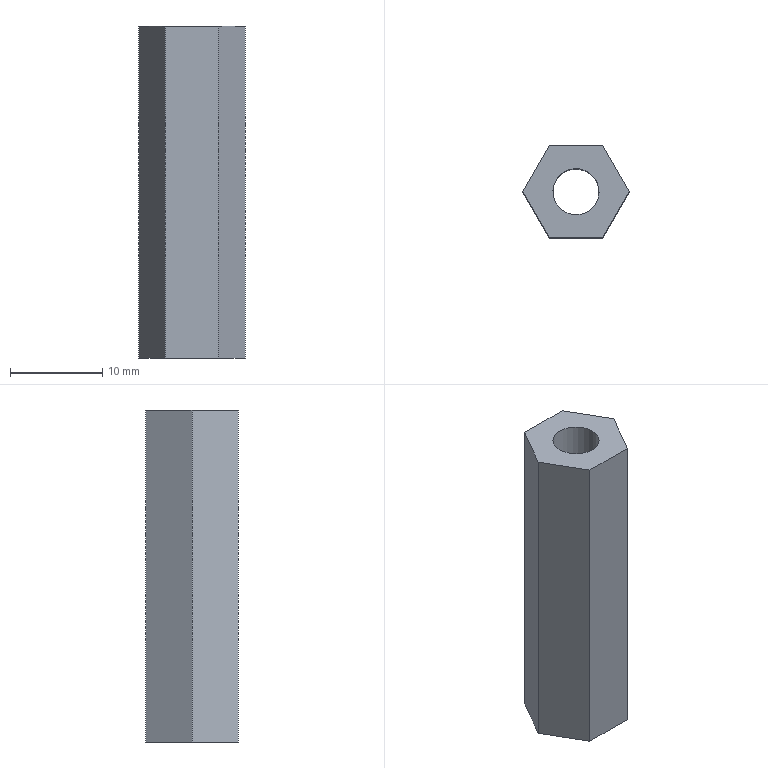Part | NX | features BREP 1 | 1 solid | 10 faces | box 11.547 x 10 x 36 mm | volume 2411 mm3 | plane 8 | cylinder 2 | commonest cylinder face diameters 5 x2
STEP:
#1=CARTESIAN_POINT('',(-121.835,201.259,18.));
#2=VERTEX_POINT('',#1);
#3=CARTESIAN_POINT('',(-126.165,203.759,18.));
#4=VERTEX_POINT('',#3);
#5=CARTESIAN_POINT('',(-124.,202.509,18.));
#6=DIRECTION('',(0.,0.,1.));
#7=DIRECTION('',(-0.866,0.5,0.));
#8=AXIS2_PLACEMENT_3D('',#5,#6,#7);
#9=CIRCLE('',#8,2.5);
#10=EDGE_CURVE('',#2,#4,#9,.T.);
#11=ORIENTED_EDGE('',*,*,#10,.T.);
#12=CARTESIAN_POINT('',(-126.165,203.759,-18.));
#13=VERTEX_POINT('',#12);
#14=CARTESIAN_POINT('',(-126.165,203.759,18.));
#15=DIRECTION('',(0.,0.,1.));
#16=VECTOR('',#15,1000.);
#17=LINE('',#14,#16);
#18=EDGE_CURVE('',#13,#4,#17,.T.);
#19=ORIENTED_EDGE('',*,*,#18,.F.);
#20=CARTESIAN_POINT('',(-121.835,201.259,-18.));
#21=VERTEX_POINT('',#20);
#22=CARTESIAN_POINT('',(-124.,202.509,-18.));
#23=DIRECTION('',(0.,0.,1.));
#24=DIRECTION('',(-0.866,0.5,0.));
#25=AXIS2_PLACEMENT_3D('',#22,#23,#24);
#26=CIRCLE('',#25,2.5);
#27=EDGE_CURVE('',#21,#13,#26,.T.);
#28=ORIENTED_EDGE('',*,*,#27,.F.);
#29=CARTESIAN_POINT('',(-121.835,201.259,18.));
#30=DIRECTION('',(0.,0.,-1.));
#31=VECTOR('',#30,1000.);
#32=LINE('',#29,#31);
#33=EDGE_CURVE('',#2,#21,#32,.T.);
#34=ORIENTED_EDGE('',*,*,#33,.F.);
#35=EDGE_LOOP('',(#11,#19,#28,#34));
#36=FACE_BOUND('',#35,.T.);
#37=CARTESIAN_POINT('',(-124.,202.509,18.));
#38=DIRECTION('',(0.,0.,-1.));
#39=DIRECTION('',(-0.866,0.5,0.));
#40=AXIS2_PLACEMENT_3D('',#37,#38,#39);
#41=CYLINDRICAL_SURFACE('',#40,2.5);
#42=ADVANCED_FACE('',(#36),#41,.F.);
#43=CARTESIAN_POINT('',(-126.887,207.509,18.));
#44=VERTEX_POINT('',#43);
#45=CARTESIAN_POINT('',(-129.774,202.509,18.));
#46=VERTEX_POINT('',#45);
#47=CARTESIAN_POINT('',(-126.887,207.509,18.));
#48=DIRECTION('',(-0.5,-0.866,0.));
#49=VECTOR('',#48,1000.);
#50=LINE('',#47,#49);
#51=EDGE_CURVE('',#44,#46,#50,.T.);
#52=ORIENTED_EDGE('',*,*,#51,.T.);
#53=CARTESIAN_POINT('',(-126.887,197.509,18.));
#54=VERTEX_POINT('',#53);
#55=CARTESIAN_POINT('',(-129.774,202.509,18.));
#56=DIRECTION('',(0.5,-0.866,0.));
#57=VECTOR('',#56,1000.);
#58=LINE('',#55,#57);
#59=EDGE_CURVE('',#46,#54,#58,.T.);
#60=ORIENTED_EDGE('',*,*,#59,.T.);
#61=CARTESIAN_POINT('',(-121.113,197.509,18.));
#62=VERTEX_POINT('',#61);
#63=CARTESIAN_POINT('',(-126.887,197.509,18.));
#64=DIRECTION('',(1.,0.,0.));
#65=VECTOR('',#64,1000.);
#66=LINE('',#63,#65);
#67=EDGE_CURVE('',#54,#62,#66,.T.);
#68=ORIENTED_EDGE('',*,*,#67,.T.);
#69=CARTESIAN_POINT('',(-118.226,202.509,18.));
#70=VERTEX_POINT('',#69);
#71=CARTESIAN_POINT('',(-121.113,197.509,18.));
#72=DIRECTION('',(0.5,0.866,0.));
#73=VECTOR('',#72,1000.);
#74=LINE('',#71,#73);
#75=EDGE_CURVE('',#62,#70,#74,.T.);
#76=ORIENTED_EDGE('',*,*,#75,.T.);
#77=CARTESIAN_POINT('',(-121.113,207.509,18.));
#78=VERTEX_POINT('',#77);
#79=CARTESIAN_POINT('',(-118.226,202.509,18.));
#80=DIRECTION('',(-0.5,0.866,0.));
#81=VECTOR('',#80,1000.);
#82=LINE('',#79,#81);
#83=EDGE_CURVE('',#70,#78,#82,.T.);
#84=ORIENTED_EDGE('',*,*,#83,.T.);
#85=CARTESIAN_POINT('',(-121.113,207.509,18.));
#86=DIRECTION('',(-1.,0.,0.));
#87=VECTOR('',#86,1000.);
#88=LINE('',#85,#87);
#89=EDGE_CURVE('',#78,#44,#88,.T.);
#90=ORIENTED_EDGE('',*,*,#89,.T.);
#91=EDGE_LOOP('',(#52,#60,#68,#76,#84,#90));
#92=FACE_BOUND('',#91,.T.);
#93=ORIENTED_EDGE('',*,*,#10,.F.);
#94=CARTESIAN_POINT('',(-124.,202.509,18.));
#95=DIRECTION('',(0.,0.,1.));
#96=DIRECTION('',(-0.866,0.5,0.));
#97=AXIS2_PLACEMENT_3D('',#94,#95,#96);
#98=CIRCLE('',#97,2.5);
#99=EDGE_CURVE('',#4,#2,#98,.T.);
#100=ORIENTED_EDGE('',*,*,#99,.F.);
#101=EDGE_LOOP('',(#93,#100));
#102=FACE_BOUND('',#101,.T.);
#103=CARTESIAN_POINT('',(-124.,202.509,18.));
#104=DIRECTION('',(0.,0.,1.));
#105=DIRECTION('',(0.866,-0.5,0.));
#106=AXIS2_PLACEMENT_3D('',#103,#104,#105);
#107=PLANE('',#106);
#108=ADVANCED_FACE('',(#92,#102),#107,.T.);
#109=CARTESIAN_POINT('',(-126.887,207.509,-18.));
#110=VERTEX_POINT('',#109);
#111=CARTESIAN_POINT('',(-129.774,202.509,-18.));
#112=VERTEX_POINT('',#111);
#113=CARTESIAN_POINT('',(-126.887,207.509,-18.));
#114=DIRECTION('',(-0.5,-0.866,0.));
#115=VECTOR('',#114,1000.);
#116=LINE('',#113,#115);
#117=EDGE_CURVE('',#110,#112,#116,.T.);
#118=ORIENTED_EDGE('',*,*,#117,.F.);
#119=CARTESIAN_POINT('',(-121.113,207.509,-18.));
#120=VERTEX_POINT('',#119);
#121=CARTESIAN_POINT('',(-121.113,207.509,-18.));
#122=DIRECTION('',(-1.,0.,0.));
#123=VECTOR('',#122,1000.);
#124=LINE('',#121,#123);
#125=EDGE_CURVE('',#120,#110,#124,.T.);
#126=ORIENTED_EDGE('',*,*,#125,.F.);
#127=CARTESIAN_POINT('',(-118.226,202.509,-18.));
#128=VERTEX_POINT('',#127);
#129=CARTESIAN_POINT('',(-118.226,202.509,-18.));
#130=DIRECTION('',(-0.5,0.866,0.));
#131=VECTOR('',#130,1000.);
#132=LINE('',#129,#131);
#133=EDGE_CURVE('',#128,#120,#132,.T.);
#134=ORIENTED_EDGE('',*,*,#133,.F.);
#135=CARTESIAN_POINT('',(-121.113,197.509,-18.));
#136=VERTEX_POINT('',#135);
#137=CARTESIAN_POINT('',(-121.113,197.509,-18.));
#138=DIRECTION('',(0.5,0.866,0.));
#139=VECTOR('',#138,1000.);
#140=LINE('',#137,#139);
#141=EDGE_CURVE('',#136,#128,#140,.T.);
#142=ORIENTED_EDGE('',*,*,#141,.F.);
#143=CARTESIAN_POINT('',(-126.887,197.509,-18.));
#144=VERTEX_POINT('',#143);
#145=CARTESIAN_POINT('',(-126.887,197.509,-18.));
#146=DIRECTION('',(1.,0.,0.));
#147=VECTOR('',#146,1000.);
#148=LINE('',#145,#147);
#149=EDGE_CURVE('',#144,#136,#148,.T.);
#150=ORIENTED_EDGE('',*,*,#149,.F.);
#151=CARTESIAN_POINT('',(-129.774,202.509,-18.));
#152=DIRECTION('',(0.5,-0.866,0.));
#153=VECTOR('',#152,1000.);
#154=LINE('',#151,#153);
#155=EDGE_CURVE('',#112,#144,#154,.T.);
#156=ORIENTED_EDGE('',*,*,#155,.F.);
#157=EDGE_LOOP('',(#118,#126,#134,#142,#150,#156));
#158=FACE_BOUND('',#157,.T.);
#159=ORIENTED_EDGE('',*,*,#27,.T.);
#160=CARTESIAN_POINT('',(-124.,202.509,-18.));
#161=DIRECTION('',(0.,0.,1.));
#162=DIRECTION('',(-0.866,0.5,0.));
#163=AXIS2_PLACEMENT_3D('',#160,#161,#162);
#164=CIRCLE('',#163,2.5);
#165=EDGE_CURVE('',#13,#21,#164,.T.);
#166=ORIENTED_EDGE('',*,*,#165,.T.);
#167=EDGE_LOOP('',(#159,#166));
#168=FACE_BOUND('',#167,.T.);
#169=CARTESIAN_POINT('',(-124.,202.509,-18.));
#170=DIRECTION('',(0.,0.,1.));
#171=DIRECTION('',(0.866,-0.5,0.));
#172=AXIS2_PLACEMENT_3D('',#169,#170,#171);
#173=PLANE('',#172);
#174=ADVANCED_FACE('',(#158,#168),#173,.F.);
#175=ORIENTED_EDGE('',*,*,#117,.T.);
#176=CARTESIAN_POINT('',(-129.774,202.509,18.));
#177=DIRECTION('',(0.,0.,-1.));
#178=VECTOR('',#177,1000.);
#179=LINE('',#176,#178);
#180=EDGE_CURVE('',#46,#112,#179,.T.);
#181=ORIENTED_EDGE('',*,*,#180,.F.);
#182=ORIENTED_EDGE('',*,*,#51,.F.);
#183=CARTESIAN_POINT('',(-126.887,207.509,18.));
#184=DIRECTION('',(0.,0.,-1.));
#185=VECTOR('',#184,1000.);
#186=LINE('',#183,#185);
#187=EDGE_CURVE('',#44,#110,#186,.T.);
#188=ORIENTED_EDGE('',*,*,#187,.T.);
#189=EDGE_LOOP('',(#175,#181,#182,#188));
#190=FACE_BOUND('',#189,.T.);
#191=CARTESIAN_POINT('',(-126.887,207.509,18.));
#192=DIRECTION('',(0.866,-0.5,0.));
#193=DIRECTION('',(-0.5,-0.866,0.));
#194=AXIS2_PLACEMENT_3D('',#191,#192,#193);
#195=PLANE('',#194);
#196=ADVANCED_FACE('',(#190),#195,.F.);
#197=ORIENTED_EDGE('',*,*,#155,.T.);
#198=CARTESIAN_POINT('',(-126.887,197.509,18.));
#199=DIRECTION('',(0.,0.,-1.));
#200=VECTOR('',#199,1000.);
#201=LINE('',#198,#200);
#202=EDGE_CURVE('',#54,#144,#201,.T.);
#203=ORIENTED_EDGE('',*,*,#202,.F.);
#204=ORIENTED_EDGE('',*,*,#59,.F.);
#205=ORIENTED_EDGE('',*,*,#180,.T.);
#206=EDGE_LOOP('',(#197,#203,#204,#205));
#207=FACE_BOUND('',#206,.T.);
#208=CARTESIAN_POINT('',(-129.774,202.509,18.));
#209=DIRECTION('',(0.866,0.5,0.));
#210=DIRECTION('',(0.5,-0.866,0.));
#211=AXIS2_PLACEMENT_3D('',#208,#209,#210);
#212=PLANE('',#211);
#213=ADVANCED_FACE('',(#207),#212,.F.);
#214=ORIENTED_EDGE('',*,*,#149,.T.);
#215=CARTESIAN_POINT('',(-121.113,197.509,18.));
#216=DIRECTION('',(0.,0.,-1.));
#217=VECTOR('',#216,1000.);
#218=LINE('',#215,#217);
#219=EDGE_CURVE('',#62,#136,#218,.T.);
#220=ORIENTED_EDGE('',*,*,#219,.F.);
#221=ORIENTED_EDGE('',*,*,#67,.F.);
#222=ORIENTED_EDGE('',*,*,#202,.T.);
#223=EDGE_LOOP('',(#214,#220,#221,#222));
#224=FACE_BOUND('',#223,.T.);
#225=CARTESIAN_POINT('',(-126.887,197.509,18.));
#226=DIRECTION('',(0.,1.,0.));
#227=DIRECTION('',(1.,0.,0.));
#228=AXIS2_PLACEMENT_3D('',#225,#226,#227);
#229=PLANE('',#228);
#230=ADVANCED_FACE('',(#224),#229,.F.);
#231=ORIENTED_EDGE('',*,*,#141,.T.);
#232=CARTESIAN_POINT('',(-118.226,202.509,18.));
#233=DIRECTION('',(0.,0.,-1.));
#234=VECTOR('',#233,1000.);
#235=LINE('',#232,#234);
#236=EDGE_CURVE('',#70,#128,#235,.T.);
#237=ORIENTED_EDGE('',*,*,#236,.F.);
#238=ORIENTED_EDGE('',*,*,#75,.F.);
#239=ORIENTED_EDGE('',*,*,#219,.T.);
#240=EDGE_LOOP('',(#231,#237,#238,#239));
#241=FACE_BOUND('',#240,.T.);
#242=CARTESIAN_POINT('',(-121.113,197.509,18.));
#243=DIRECTION('',(-0.866,0.5,0.));
#244=DIRECTION('',(0.5,0.866,0.));
#245=AXIS2_PLACEMENT_3D('',#242,#243,#244);
#246=PLANE('',#245);
#247=ADVANCED_FACE('',(#241),#246,.F.);
#248=ORIENTED_EDGE('',*,*,#133,.T.);
#249=CARTESIAN_POINT('',(-121.113,207.509,18.));
#250=DIRECTION('',(0.,0.,-1.));
#251=VECTOR('',#250,1000.);
#252=LINE('',#249,#251);
#253=EDGE_CURVE('',#78,#120,#252,.T.);
#254=ORIENTED_EDGE('',*,*,#253,.F.);
#255=ORIENTED_EDGE('',*,*,#83,.F.);
#256=ORIENTED_EDGE('',*,*,#236,.T.);
#257=EDGE_LOOP('',(#248,#254,#255,#256));
#258=FACE_BOUND('',#257,.T.);
#259=CARTESIAN_POINT('',(-118.226,202.509,18.));
#260=DIRECTION('',(-0.866,-0.5,0.));
#261=DIRECTION('',(-0.5,0.866,0.));
#262=AXIS2_PLACEMENT_3D('',#259,#260,#261);
#263=PLANE('',#262);
#264=ADVANCED_FACE('',(#258),#263,.F.);
#265=ORIENTED_EDGE('',*,*,#125,.T.);
#266=ORIENTED_EDGE('',*,*,#187,.F.);
#267=ORIENTED_EDGE('',*,*,#89,.F.);
#268=ORIENTED_EDGE('',*,*,#253,.T.);
#269=EDGE_LOOP('',(#265,#266,#267,#268));
#270=FACE_BOUND('',#269,.T.);
#271=CARTESIAN_POINT('',(-121.113,207.509,18.));
#272=DIRECTION('',(0.,-1.,0.));
#273=DIRECTION('',(-1.,0.,0.));
#274=AXIS2_PLACEMENT_3D('',#271,#272,#273);
#275=PLANE('',#274);
#276=ADVANCED_FACE('',(#270),#275,.F.);
#277=ORIENTED_EDGE('',*,*,#18,.T.);
#278=ORIENTED_EDGE('',*,*,#99,.T.);
#279=ORIENTED_EDGE('',*,*,#33,.T.);
#280=ORIENTED_EDGE('',*,*,#165,.F.);
#281=EDGE_LOOP('',(#277,#278,#279,#280));
#282=FACE_BOUND('',#281,.T.);
#283=CARTESIAN_POINT('',(-124.,202.509,18.));
#284=DIRECTION('',(0.,0.,-1.));
#285=DIRECTION('',(-0.866,0.5,0.));
#286=AXIS2_PLACEMENT_3D('',#283,#284,#285);
#287=CYLINDRICAL_SURFACE('',#286,2.5);
#288=ADVANCED_FACE('',(#282),#287,.F.);
#289=CLOSED_SHELL('',(#42,#108,#174,#196,#213,#230,#247,#264,#276,#288));
#290=MANIFOLD_SOLID_BREP('',#289);
#291=(LENGTH_UNIT()NAMED_UNIT(*)SI_UNIT(.MILLI.,.METRE.));
#292=UNCERTAINTY_MEASURE_WITH_UNIT(LENGTH_MEASURE(0.00001),#291,'','');
#293=(NAMED_UNIT(*)PLANE_ANGLE_UNIT()SI_UNIT($,.RADIAN.));
#294=(NAMED_UNIT(*)SI_UNIT($,.STERADIAN.)SOLID_ANGLE_UNIT());
#295=(GEOMETRIC_REPRESENTATION_CONTEXT(3)GLOBAL_UNCERTAINTY_ASSIGNED_CONTEXT((#292))GLOBAL_UNIT_ASSIGNED_CONTEXT((#291,#293,#294))REPRESENTATION_CONTEXT('',''));
#296=ADVANCED_BREP_SHAPE_REPRESENTATION('',(#290),#295);